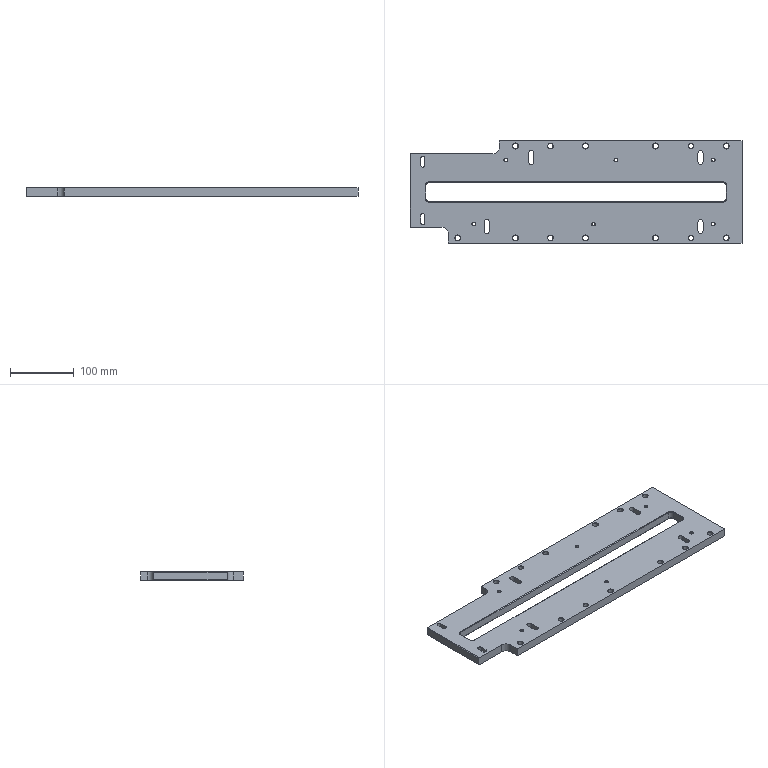Part | STEP file | Tube feed_id1774_x_t | 1 solid | 119 faces | box 520 x 160 x 13.5 mm | volume 851655 mm3 | cone 46 | cylinder 37 | plane 36 | commonest cylinder face diameters 8.5 x9 8 x8 5 x6 6.8 x4 8.02 x4 10 x4